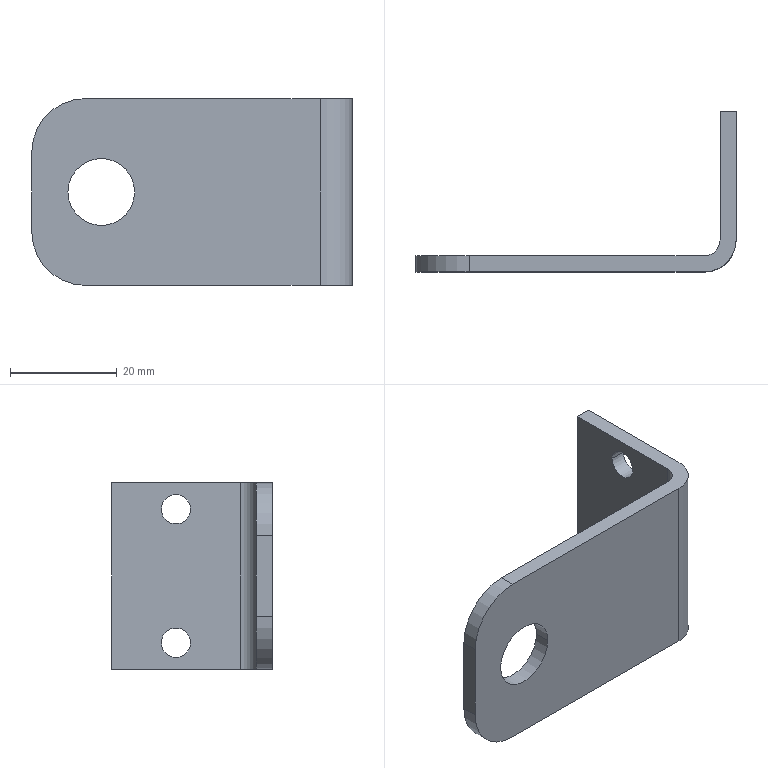Part | STEP file | X77-04022 | 1 solid | 18 faces | box 60 x 30 x 35 mm | volume 8293 mm3 | cylinder 10 | plane 8 | commonest cylinder face diameters 5.5 x4 12.5 x2 20 x2 6 x1 12 x1
STEP:
#1=CARTESIAN_POINT('',(-37.75,-30.,17.5));
#2=VERTEX_POINT('',#1);
#3=CARTESIAN_POINT('',(-50.25,-30.,17.5));
#4=VERTEX_POINT('',#3);
#5=CARTESIAN_POINT('',(-44.,-30.,17.5));
#6=DIRECTION('',(0.,1.,0.));
#7=DIRECTION('',(-1.,0.,0.));
#8=AXIS2_PLACEMENT_3D('',#5,#6,#7);
#9=CIRCLE('',#8,6.25);
#10=EDGE_CURVE('',#2,#4,#9,.T.);
#11=ORIENTED_EDGE('',*,*,#10,.F.);
#12=CARTESIAN_POINT('',(-37.75,-27.,17.5));
#13=VERTEX_POINT('',#12);
#14=CARTESIAN_POINT('',(-37.75,-30.,17.5));
#15=DIRECTION('',(0.,1.,0.));
#16=VECTOR('',#15,1000.);
#17=LINE('',#14,#16);
#18=EDGE_CURVE('',#2,#13,#17,.T.);
#19=ORIENTED_EDGE('',*,*,#18,.T.);
#20=CARTESIAN_POINT('',(-50.25,-27.,17.5));
#21=VERTEX_POINT('',#20);
#22=CARTESIAN_POINT('',(-44.,-27.,17.5));
#23=DIRECTION('',(0.,1.,0.));
#24=DIRECTION('',(-1.,0.,0.));
#25=AXIS2_PLACEMENT_3D('',#22,#23,#24);
#26=CIRCLE('',#25,6.25);
#27=EDGE_CURVE('',#13,#21,#26,.T.);
#28=ORIENTED_EDGE('',*,*,#27,.T.);
#29=CARTESIAN_POINT('',(-50.25,-30.,17.5));
#30=DIRECTION('',(0.,1.,0.));
#31=VECTOR('',#30,1000.);
#32=LINE('',#29,#31);
#33=EDGE_CURVE('',#4,#21,#32,.T.);
#34=ORIENTED_EDGE('',*,*,#33,.F.);
#35=EDGE_LOOP('',(#11,#19,#28,#34));
#36=FACE_OUTER_BOUND('',#35,.T.);
#37=CARTESIAN_POINT('',(-44.,-30.,17.5));
#38=DIRECTION('',(0.,1.,0.));
#39=DIRECTION('',(-1.,0.,0.));
#40=AXIS2_PLACEMENT_3D('',#37,#38,#39);
#41=CYLINDRICAL_SURFACE('',#40,6.25);
#42=ADVANCED_FACE('',(#36),#41,.F.);
#43=CARTESIAN_POINT('',(3.,-9.25,30.));
#44=VERTEX_POINT('',#43);
#45=CARTESIAN_POINT('',(3.,-14.75,30.));
#46=VERTEX_POINT('',#45);
#47=CARTESIAN_POINT('',(3.,-12.,30.));
#48=DIRECTION('',(-1.,0.,0.));
#49=DIRECTION('',(0.,-1.,0.));
#50=AXIS2_PLACEMENT_3D('',#47,#48,#49);
#51=CIRCLE('',#50,2.75);
#52=EDGE_CURVE('',#44,#46,#51,.T.);
#53=ORIENTED_EDGE('',*,*,#52,.F.);
#54=CARTESIAN_POINT('',(0.,-9.25,30.));
#55=VERTEX_POINT('',#54);
#56=CARTESIAN_POINT('',(3.,-9.25,30.));
#57=DIRECTION('',(-1.,0.,0.));
#58=VECTOR('',#57,1000.);
#59=LINE('',#56,#58);
#60=EDGE_CURVE('',#44,#55,#59,.T.);
#61=ORIENTED_EDGE('',*,*,#60,.T.);
#62=CARTESIAN_POINT('',(0.,-14.75,30.));
#63=VERTEX_POINT('',#62);
#64=CARTESIAN_POINT('',(0.,-12.,30.));
#65=DIRECTION('',(-1.,0.,0.));
#66=DIRECTION('',(0.,-1.,0.));
#67=AXIS2_PLACEMENT_3D('',#64,#65,#66);
#68=CIRCLE('',#67,2.75);
#69=EDGE_CURVE('',#55,#63,#68,.T.);
#70=ORIENTED_EDGE('',*,*,#69,.T.);
#71=CARTESIAN_POINT('',(3.,-14.75,30.));
#72=DIRECTION('',(-1.,0.,0.));
#73=VECTOR('',#72,1000.);
#74=LINE('',#71,#73);
#75=EDGE_CURVE('',#46,#63,#74,.T.);
#76=ORIENTED_EDGE('',*,*,#75,.F.);
#77=EDGE_LOOP('',(#53,#61,#70,#76));
#78=FACE_OUTER_BOUND('',#77,.T.);
#79=CARTESIAN_POINT('',(3.,-12.,30.));
#80=DIRECTION('',(-1.,0.,0.));
#81=DIRECTION('',(0.,-1.,0.));
#82=AXIS2_PLACEMENT_3D('',#79,#80,#81);
#83=CYLINDRICAL_SURFACE('',#82,2.75);
#84=ADVANCED_FACE('',(#78),#83,.F.);
#85=CARTESIAN_POINT('',(3.,-9.25,5.));
#86=VERTEX_POINT('',#85);
#87=CARTESIAN_POINT('',(3.,-14.75,5.));
#88=VERTEX_POINT('',#87);
#89=CARTESIAN_POINT('',(3.,-12.,5.));
#90=DIRECTION('',(-1.,0.,0.));
#91=DIRECTION('',(0.,-1.,0.));
#92=AXIS2_PLACEMENT_3D('',#89,#90,#91);
#93=CIRCLE('',#92,2.75);
#94=EDGE_CURVE('',#86,#88,#93,.T.);
#95=ORIENTED_EDGE('',*,*,#94,.F.);
#96=CARTESIAN_POINT('',(0.,-9.25,5.));
#97=VERTEX_POINT('',#96);
#98=CARTESIAN_POINT('',(3.,-9.25,5.));
#99=DIRECTION('',(-1.,0.,0.));
#100=VECTOR('',#99,1000.);
#101=LINE('',#98,#100);
#102=EDGE_CURVE('',#86,#97,#101,.T.);
#103=ORIENTED_EDGE('',*,*,#102,.T.);
#104=CARTESIAN_POINT('',(0.,-14.75,5.));
#105=VERTEX_POINT('',#104);
#106=CARTESIAN_POINT('',(0.,-12.,5.));
#107=DIRECTION('',(-1.,0.,0.));
#108=DIRECTION('',(0.,-1.,0.));
#109=AXIS2_PLACEMENT_3D('',#106,#107,#108);
#110=CIRCLE('',#109,2.75);
#111=EDGE_CURVE('',#97,#105,#110,.T.);
#112=ORIENTED_EDGE('',*,*,#111,.T.);
#113=CARTESIAN_POINT('',(3.,-14.75,5.));
#114=DIRECTION('',(-1.,0.,0.));
#115=VECTOR('',#114,1000.);
#116=LINE('',#113,#115);
#117=EDGE_CURVE('',#88,#105,#116,.T.);
#118=ORIENTED_EDGE('',*,*,#117,.F.);
#119=EDGE_LOOP('',(#95,#103,#112,#118));
#120=FACE_OUTER_BOUND('',#119,.T.);
#121=CARTESIAN_POINT('',(3.,-12.,5.));
#122=DIRECTION('',(-1.,0.,0.));
#123=DIRECTION('',(0.,-1.,0.));
#124=AXIS2_PLACEMENT_3D('',#121,#122,#123);
#125=CYLINDRICAL_SURFACE('',#124,2.75);
#126=ADVANCED_FACE('',(#120),#125,.F.);
#127=CARTESIAN_POINT('',(3.,0.,0.));
#128=VERTEX_POINT('',#127);
#129=CARTESIAN_POINT('',(0.,0.,0.));
#130=VERTEX_POINT('',#129);
#131=CARTESIAN_POINT('',(3.,0.,0.));
#132=DIRECTION('',(-1.,0.,0.));
#133=VECTOR('',#132,1000.);
#134=LINE('',#131,#133);
#135=EDGE_CURVE('',#128,#130,#134,.T.);
#136=ORIENTED_EDGE('',*,*,#135,.T.);
#137=CARTESIAN_POINT('',(0.,0.,35.));
#138=VERTEX_POINT('',#137);
#139=CARTESIAN_POINT('',(0.,0.,35.));
#140=DIRECTION('',(0.,0.,-1.));
#141=VECTOR('',#140,1000.);
#142=LINE('',#139,#141);
#143=EDGE_CURVE('',#138,#130,#142,.T.);
#144=ORIENTED_EDGE('',*,*,#143,.F.);
#145=CARTESIAN_POINT('',(3.,0.,35.));
#146=VERTEX_POINT('',#145);
#147=CARTESIAN_POINT('',(3.,0.,35.));
#148=DIRECTION('',(-1.,0.,0.));
#149=VECTOR('',#148,1000.);
#150=LINE('',#147,#149);
#151=EDGE_CURVE('',#146,#138,#150,.T.);
#152=ORIENTED_EDGE('',*,*,#151,.F.);
#153=CARTESIAN_POINT('',(3.,0.,35.));
#154=DIRECTION('',(0.,0.,-1.));
#155=VECTOR('',#154,1000.);
#156=LINE('',#153,#155);
#157=EDGE_CURVE('',#146,#128,#156,.T.);
#158=ORIENTED_EDGE('',*,*,#157,.T.);
#159=EDGE_LOOP('',(#136,#144,#152,#158));
#160=FACE_OUTER_BOUND('',#159,.T.);
#161=CARTESIAN_POINT('',(3.,0.,35.));
#162=DIRECTION('',(0.,-1.,0.));
#163=DIRECTION('',(1.,0.,0.));
#164=AXIS2_PLACEMENT_3D('',#161,#162,#163);
#165=PLANE('',#164);
#166=ADVANCED_FACE('',(#160),#165,.F.);
#167=CARTESIAN_POINT('',(0.,-12.,30.));
#168=DIRECTION('',(-1.,0.,0.));
#169=DIRECTION('',(0.,-1.,0.));
#170=AXIS2_PLACEMENT_3D('',#167,#168,#169);
#171=CIRCLE('',#170,2.75);
#172=EDGE_CURVE('',#63,#55,#171,.T.);
#173=ORIENTED_EDGE('',*,*,#172,.F.);
#174=ORIENTED_EDGE('',*,*,#69,.F.);
#175=EDGE_LOOP('',(#173,#174));
#176=FACE_BOUND('',#175,.T.);
#177=CARTESIAN_POINT('',(0.,-12.,5.));
#178=DIRECTION('',(-1.,0.,0.));
#179=DIRECTION('',(0.,-1.,0.));
#180=AXIS2_PLACEMENT_3D('',#177,#178,#179);
#181=CIRCLE('',#180,2.75);
#182=EDGE_CURVE('',#105,#97,#181,.T.);
#183=ORIENTED_EDGE('',*,*,#182,.F.);
#184=ORIENTED_EDGE('',*,*,#111,.F.);
#185=EDGE_LOOP('',(#183,#184));
#186=FACE_BOUND('',#185,.T.);
#187=CARTESIAN_POINT('',(0.,-24.,0.));
#188=VERTEX_POINT('',#187);
#189=CARTESIAN_POINT('',(0.,0.,0.));
#190=DIRECTION('',(0.,-1.,0.));
#191=VECTOR('',#190,1000.);
#192=LINE('',#189,#191);
#193=EDGE_CURVE('',#130,#188,#192,.T.);
#194=ORIENTED_EDGE('',*,*,#193,.T.);
#195=CARTESIAN_POINT('',(0.,-24.,35.));
#196=VERTEX_POINT('',#195);
#197=CARTESIAN_POINT('',(0.,-24.,35.));
#198=DIRECTION('',(0.,0.,-1.));
#199=VECTOR('',#198,1000.);
#200=LINE('',#197,#199);
#201=EDGE_CURVE('',#196,#188,#200,.T.);
#202=ORIENTED_EDGE('',*,*,#201,.F.);
#203=CARTESIAN_POINT('',(0.,0.,35.));
#204=DIRECTION('',(0.,-1.,0.));
#205=VECTOR('',#204,1000.);
#206=LINE('',#203,#205);
#207=EDGE_CURVE('',#138,#196,#206,.T.);
#208=ORIENTED_EDGE('',*,*,#207,.F.);
#209=ORIENTED_EDGE('',*,*,#143,.T.);
#210=EDGE_LOOP('',(#194,#202,#208,#209));
#211=FACE_OUTER_BOUND('',#210,.T.);
#212=CARTESIAN_POINT('',(0.,0.,35.));
#213=DIRECTION('',(1.,0.,0.));
#214=DIRECTION('',(0.,1.,0.));
#215=AXIS2_PLACEMENT_3D('',#212,#213,#214);
#216=PLANE('',#215);
#217=ADVANCED_FACE('',(#176,#186,#211),#216,.F.);
#218=CARTESIAN_POINT('',(-3.,-27.,0.));
#219=VERTEX_POINT('',#218);
#220=CARTESIAN_POINT('',(-3.,-24.,0.));
#221=DIRECTION('',(0.,0.,-1.));
#222=DIRECTION('',(1.,0.,0.));
#223=AXIS2_PLACEMENT_3D('',#220,#221,#222);
#224=CIRCLE('',#223,3.);
#225=EDGE_CURVE('',#188,#219,#224,.T.);
#226=ORIENTED_EDGE('',*,*,#225,.T.);
#227=CARTESIAN_POINT('',(-3.,-27.,35.));
#228=VERTEX_POINT('',#227);
#229=CARTESIAN_POINT('',(-3.,-27.,35.));
#230=DIRECTION('',(0.,0.,-1.));
#231=VECTOR('',#230,1000.);
#232=LINE('',#229,#231);
#233=EDGE_CURVE('',#228,#219,#232,.T.);
#234=ORIENTED_EDGE('',*,*,#233,.F.);
#235=CARTESIAN_POINT('',(-3.,-24.,35.));
#236=DIRECTION('',(0.,0.,-1.));
#237=DIRECTION('',(1.,0.,0.));
#238=AXIS2_PLACEMENT_3D('',#235,#236,#237);
#239=CIRCLE('',#238,3.);
#240=EDGE_CURVE('',#196,#228,#239,.T.);
#241=ORIENTED_EDGE('',*,*,#240,.F.);
#242=ORIENTED_EDGE('',*,*,#201,.T.);
#243=EDGE_LOOP('',(#226,#234,#241,#242));
#244=FACE_OUTER_BOUND('',#243,.T.);
#245=CARTESIAN_POINT('',(-3.,-24.,35.));
#246=DIRECTION('',(0.,0.,-1.));
#247=DIRECTION('',(-1.,0.,0.));
#248=AXIS2_PLACEMENT_3D('',#245,#246,#247);
#249=CYLINDRICAL_SURFACE('',#248,3.);
#250=ADVANCED_FACE('',(#244),#249,.F.);
#251=CARTESIAN_POINT('',(-44.,-27.,17.5));
#252=DIRECTION('',(0.,1.,0.));
#253=DIRECTION('',(-1.,0.,0.));
#254=AXIS2_PLACEMENT_3D('',#251,#252,#253);
#255=CIRCLE('',#254,6.25);
#256=EDGE_CURVE('',#21,#13,#255,.T.);
#257=ORIENTED_EDGE('',*,*,#256,.F.);
#258=ORIENTED_EDGE('',*,*,#27,.F.);
#259=EDGE_LOOP('',(#257,#258));
#260=FACE_BOUND('',#259,.T.);
#261=CARTESIAN_POINT('',(-57.,-27.,25.));
#262=VERTEX_POINT('',#261);
#263=CARTESIAN_POINT('',(-57.,-27.,10.));
#264=VERTEX_POINT('',#263);
#265=CARTESIAN_POINT('',(-57.,-27.,35.));
#266=DIRECTION('',(0.,0.,-1.));
#267=VECTOR('',#266,1000.);
#268=LINE('',#265,#267);
#269=EDGE_CURVE('',#262,#264,#268,.T.);
#270=ORIENTED_EDGE('',*,*,#269,.F.);
#271=CARTESIAN_POINT('',(-47.,-27.,35.));
#272=VERTEX_POINT('',#271);
#273=CARTESIAN_POINT('',(-47.,-27.,25.));
#274=DIRECTION('',(0.,1.,0.));
#275=DIRECTION('',(0.,0.,-1.));
#276=AXIS2_PLACEMENT_3D('',#273,#274,#275);
#277=CIRCLE('',#276,10.);
#278=EDGE_CURVE('',#262,#272,#277,.T.);
#279=ORIENTED_EDGE('',*,*,#278,.T.);
#280=CARTESIAN_POINT('',(-3.,-27.,35.));
#281=DIRECTION('',(-1.,0.,0.));
#282=VECTOR('',#281,1000.);
#283=LINE('',#280,#282);
#284=EDGE_CURVE('',#228,#272,#283,.T.);
#285=ORIENTED_EDGE('',*,*,#284,.F.);
#286=ORIENTED_EDGE('',*,*,#233,.T.);
#287=CARTESIAN_POINT('',(-47.,-27.,0.));
#288=VERTEX_POINT('',#287);
#289=CARTESIAN_POINT('',(-3.,-27.,0.));
#290=DIRECTION('',(-1.,0.,0.));
#291=VECTOR('',#290,1000.);
#292=LINE('',#289,#291);
#293=EDGE_CURVE('',#219,#288,#292,.T.);
#294=ORIENTED_EDGE('',*,*,#293,.T.);
#295=CARTESIAN_POINT('',(-47.,-27.,10.));
#296=DIRECTION('',(0.,1.,0.));
#297=DIRECTION('',(0.,0.,-1.));
#298=AXIS2_PLACEMENT_3D('',#295,#296,#297);
#299=CIRCLE('',#298,10.);
#300=EDGE_CURVE('',#288,#264,#299,.T.);
#301=ORIENTED_EDGE('',*,*,#300,.T.);
#302=EDGE_LOOP('',(#270,#279,#285,#286,#294,#301));
#303=FACE_OUTER_BOUND('',#302,.T.);
#304=CARTESIAN_POINT('',(-3.,-27.,35.));
#305=DIRECTION('',(0.,-1.,0.));
#306=DIRECTION('',(0.,0.,-1.));
#307=AXIS2_PLACEMENT_3D('',#304,#305,#306);
#308=PLANE('',#307);
#309=ADVANCED_FACE('',(#260,#303),#308,.F.);
#310=CARTESIAN_POINT('',(-57.,-30.,25.));
#311=VERTEX_POINT('',#310);
#312=CARTESIAN_POINT('',(-57.,-30.,10.));
#313=VERTEX_POINT('',#312);
#314=CARTESIAN_POINT('',(-57.,-30.,35.));
#315=DIRECTION('',(0.,0.,-1.));
#316=VECTOR('',#315,1000.);
#317=LINE('',#314,#316);
#318=EDGE_CURVE('',#311,#313,#317,.T.);
#319=ORIENTED_EDGE('',*,*,#318,.F.);
#320=CARTESIAN_POINT('',(-57.,-27.,25.));
#321=DIRECTION('',(0.,1.,0.));
#322=VECTOR('',#321,1000.);
#323=LINE('',#320,#322);
#324=EDGE_CURVE('',#311,#262,#323,.T.);
#325=ORIENTED_EDGE('',*,*,#324,.T.);
#326=ORIENTED_EDGE('',*,*,#269,.T.);
#327=CARTESIAN_POINT('',(-57.,-27.,10.));
#328=DIRECTION('',(0.,-1.,0.));
#329=VECTOR('',#328,1000.);
#330=LINE('',#327,#329);
#331=EDGE_CURVE('',#264,#313,#330,.T.);
#332=ORIENTED_EDGE('',*,*,#331,.T.);
#333=EDGE_LOOP('',(#319,#325,#326,#332));
#334=FACE_OUTER_BOUND('',#333,.T.);
#335=CARTESIAN_POINT('',(-57.,-27.,35.));
#336=DIRECTION('',(1.,0.,0.));
#337=DIRECTION('',(0.,0.,-1.));
#338=AXIS2_PLACEMENT_3D('',#335,#336,#337);
#339=PLANE('',#338);
#340=ADVANCED_FACE('',(#334),#339,.F.);
#341=CARTESIAN_POINT('',(-44.,-30.,17.5));
#342=DIRECTION('',(0.,1.,0.));
#343=DIRECTION('',(-1.,0.,0.));
#344=AXIS2_PLACEMENT_3D('',#341,#342,#343);
#345=CIRCLE('',#344,6.25);
#346=EDGE_CURVE('',#4,#2,#345,.T.);
#347=ORIENTED_EDGE('',*,*,#346,.T.);
#348=ORIENTED_EDGE('',*,*,#10,.T.);
#349=EDGE_LOOP('',(#347,#348));
#350=FACE_BOUND('',#349,.T.);
#351=CARTESIAN_POINT('',(-47.,-30.,35.));
#352=VERTEX_POINT('',#351);
#353=CARTESIAN_POINT('',(-3.,-30.,35.));
#354=VERTEX_POINT('',#353);
#355=CARTESIAN_POINT('',(-57.,-30.,35.));
#356=DIRECTION('',(1.,0.,0.));
#357=VECTOR('',#356,1000.);
#358=LINE('',#355,#357);
#359=EDGE_CURVE('',#352,#354,#358,.T.);
#360=ORIENTED_EDGE('',*,*,#359,.F.);
#361=CARTESIAN_POINT('',(-47.,-30.,25.));
#362=DIRECTION('',(0.,-1.,0.));
#363=DIRECTION('',(0.,0.,1.));
#364=AXIS2_PLACEMENT_3D('',#361,#362,#363);
#365=CIRCLE('',#364,10.);
#366=EDGE_CURVE('',#352,#311,#365,.T.);
#367=ORIENTED_EDGE('',*,*,#366,.T.);
#368=ORIENTED_EDGE('',*,*,#318,.T.);
#369=CARTESIAN_POINT('',(-47.,-30.,0.));
#370=VERTEX_POINT('',#369);
#371=CARTESIAN_POINT('',(-47.,-30.,10.));
#372=DIRECTION('',(0.,-1.,0.));
#373=DIRECTION('',(0.,0.,1.));
#374=AXIS2_PLACEMENT_3D('',#371,#372,#373);
#375=CIRCLE('',#374,10.);
#376=EDGE_CURVE('',#313,#370,#375,.T.);
#377=ORIENTED_EDGE('',*,*,#376,.T.);
#378=CARTESIAN_POINT('',(-3.,-30.,0.));
#379=VERTEX_POINT('',#378);
#380=CARTESIAN_POINT('',(-57.,-30.,0.));
#381=DIRECTION('',(1.,0.,0.));
#382=VECTOR('',#381,1000.);
#383=LINE('',#380,#382);
#384=EDGE_CURVE('',#370,#379,#383,.T.);
#385=ORIENTED_EDGE('',*,*,#384,.T.);
#386=CARTESIAN_POINT('',(-3.,-30.,35.));
#387=DIRECTION('',(0.,0.,-1.));
#388=VECTOR('',#387,1000.);
#389=LINE('',#386,#388);
#390=EDGE_CURVE('',#354,#379,#389,.T.);
#391=ORIENTED_EDGE('',*,*,#390,.F.);
#392=EDGE_LOOP('',(#360,#367,#368,#377,#385,#391));
#393=FACE_OUTER_BOUND('',#392,.T.);
#394=CARTESIAN_POINT('',(-57.,-30.,35.));
#395=DIRECTION('',(0.,1.,0.));
#396=DIRECTION('',(0.,0.,1.));
#397=AXIS2_PLACEMENT_3D('',#394,#395,#396);
#398=PLANE('',#397);
#399=ADVANCED_FACE('',(#350,#393),#398,.F.);
#400=CARTESIAN_POINT('',(3.,-24.,0.));
#401=VERTEX_POINT('',#400);
#402=CARTESIAN_POINT('',(-3.,-24.,0.));
#403=DIRECTION('',(0.,0.,1.));
#404=DIRECTION('',(1.,0.,0.));
#405=AXIS2_PLACEMENT_3D('',#402,#403,#404);
#406=CIRCLE('',#405,6.);
#407=EDGE_CURVE('',#379,#401,#406,.T.);
#408=ORIENTED_EDGE('',*,*,#407,.T.);
#409=CARTESIAN_POINT('',(3.,-24.,35.));
#410=VERTEX_POINT('',#409);
#411=CARTESIAN_POINT('',(3.,-24.,35.));
#412=DIRECTION('',(0.,0.,-1.));
#413=VECTOR('',#412,1000.);
#414=LINE('',#411,#413);
#415=EDGE_CURVE('',#410,#401,#414,.T.);
#416=ORIENTED_EDGE('',*,*,#415,.F.);
#417=CARTESIAN_POINT('',(-3.,-24.,35.));
#418=DIRECTION('',(0.,0.,1.));
#419=DIRECTION('',(1.,0.,0.));
#420=AXIS2_PLACEMENT_3D('',#417,#418,#419);
#421=CIRCLE('',#420,6.);
#422=EDGE_CURVE('',#354,#410,#421,.T.);
#423=ORIENTED_EDGE('',*,*,#422,.F.);
#424=ORIENTED_EDGE('',*,*,#390,.T.);
#425=EDGE_LOOP('',(#408,#416,#423,#424));
#426=FACE_OUTER_BOUND('',#425,.T.);
#427=CARTESIAN_POINT('',(-3.,-24.,35.));
#428=DIRECTION('',(0.,0.,-1.));
#429=DIRECTION('',(-1.,0.,0.));
#430=AXIS2_PLACEMENT_3D('',#427,#428,#429);
#431=CYLINDRICAL_SURFACE('',#430,6.);
#432=ADVANCED_FACE('',(#426),#431,.T.);
#433=CARTESIAN_POINT('',(3.,-12.,30.));
#434=DIRECTION('',(-1.,0.,0.));
#435=DIRECTION('',(0.,-1.,0.));
#436=AXIS2_PLACEMENT_3D('',#433,#434,#435);
#437=CIRCLE('',#436,2.75);
#438=EDGE_CURVE('',#46,#44,#437,.T.);
#439=ORIENTED_EDGE('',*,*,#438,.T.);
#440=ORIENTED_EDGE('',*,*,#52,.T.);
#441=EDGE_LOOP('',(#439,#440));
#442=FACE_BOUND('',#441,.T.);
#443=CARTESIAN_POINT('',(3.,-12.,5.));
#444=DIRECTION('',(-1.,0.,0.));
#445=DIRECTION('',(0.,-1.,0.));
#446=AXIS2_PLACEMENT_3D('',#443,#444,#445);
#447=CIRCLE('',#446,2.75);
#448=EDGE_CURVE('',#88,#86,#447,.T.);
#449=ORIENTED_EDGE('',*,*,#448,.T.);
#450=ORIENTED_EDGE('',*,*,#94,.T.);
#451=EDGE_LOOP('',(#449,#450));
#452=FACE_BOUND('',#451,.T.);
#453=CARTESIAN_POINT('',(3.,-24.,0.));
#454=DIRECTION('',(0.,1.,0.));
#455=VECTOR('',#454,1000.);
#456=LINE('',#453,#455);
#457=EDGE_CURVE('',#401,#128,#456,.T.);
#458=ORIENTED_EDGE('',*,*,#457,.T.);
#459=ORIENTED_EDGE('',*,*,#157,.F.);
#460=CARTESIAN_POINT('',(3.,-24.,35.));
#461=DIRECTION('',(0.,1.,0.));
#462=VECTOR('',#461,1000.);
#463=LINE('',#460,#462);
#464=EDGE_CURVE('',#410,#146,#463,.T.);
#465=ORIENTED_EDGE('',*,*,#464,.F.);
#466=ORIENTED_EDGE('',*,*,#415,.T.);
#467=EDGE_LOOP('',(#458,#459,#465,#466));
#468=FACE_OUTER_BOUND('',#467,.T.);
#469=CARTESIAN_POINT('',(3.,-24.,35.));
#470=DIRECTION('',(-1.,0.,0.));
#471=DIRECTION('',(0.,0.,1.));
#472=AXIS2_PLACEMENT_3D('',#469,#470,#471);
#473=PLANE('',#472);
#474=ADVANCED_FACE('',(#442,#452,#468),#473,.F.);
#475=ORIENTED_EDGE('',*,*,#284,.T.);
#476=CARTESIAN_POINT('',(-47.,-30.,35.));
#477=DIRECTION('',(0.,-1.,0.));
#478=VECTOR('',#477,1000.);
#479=LINE('',#476,#478);
#480=EDGE_CURVE('',#272,#352,#479,.T.);
#481=ORIENTED_EDGE('',*,*,#480,.T.);
#482=ORIENTED_EDGE('',*,*,#359,.T.);
#483=ORIENTED_EDGE('',*,*,#422,.T.);
#484=ORIENTED_EDGE('',*,*,#464,.T.);
#485=ORIENTED_EDGE('',*,*,#151,.T.);
#486=ORIENTED_EDGE('',*,*,#207,.T.);
#487=ORIENTED_EDGE('',*,*,#240,.T.);
#488=EDGE_LOOP('',(#475,#481,#482,#483,#484,#485,#486,#487));
#489=FACE_OUTER_BOUND('',#488,.T.);
#490=CARTESIAN_POINT('',(-3.,-24.,35.));
#491=DIRECTION('',(0.,0.,1.));
#492=DIRECTION('',(1.,0.,0.));
#493=AXIS2_PLACEMENT_3D('',#490,#491,#492);
#494=PLANE('',#493);
#495=ADVANCED_FACE('',(#489),#494,.T.);
#496=ORIENTED_EDGE('',*,*,#384,.F.);
#497=CARTESIAN_POINT('',(-47.,-24.,0.));
#498=DIRECTION('',(0.,1.,0.));
#499=VECTOR('',#498,1000.);
#500=LINE('',#497,#499);
#501=EDGE_CURVE('',#370,#288,#500,.T.);
#502=ORIENTED_EDGE('',*,*,#501,.T.);
#503=ORIENTED_EDGE('',*,*,#293,.F.);
#504=ORIENTED_EDGE('',*,*,#225,.F.);
#505=ORIENTED_EDGE('',*,*,#193,.F.);
#506=ORIENTED_EDGE('',*,*,#135,.F.);
#507=ORIENTED_EDGE('',*,*,#457,.F.);
#508=ORIENTED_EDGE('',*,*,#407,.F.);
#509=EDGE_LOOP('',(#496,#502,#503,#504,#505,#506,#507,#508));
#510=FACE_OUTER_BOUND('',#509,.T.);
#511=CARTESIAN_POINT('',(-3.,-24.,0.));
#512=DIRECTION('',(0.,0.,1.));
#513=DIRECTION('',(1.,0.,0.));
#514=AXIS2_PLACEMENT_3D('',#511,#512,#513);
#515=PLANE('',#514);
#516=ADVANCED_FACE('',(#510),#515,.F.);
#517=ORIENTED_EDGE('',*,*,#102,.F.);
#518=ORIENTED_EDGE('',*,*,#448,.F.);
#519=ORIENTED_EDGE('',*,*,#117,.T.);
#520=ORIENTED_EDGE('',*,*,#182,.T.);
#521=EDGE_LOOP('',(#517,#518,#519,#520));
#522=FACE_OUTER_BOUND('',#521,.T.);
#523=CARTESIAN_POINT('',(3.,-12.,5.));
#524=DIRECTION('',(-1.,0.,0.));
#525=DIRECTION('',(0.,-1.,0.));
#526=AXIS2_PLACEMENT_3D('',#523,#524,#525);
#527=CYLINDRICAL_SURFACE('',#526,2.75);
#528=ADVANCED_FACE('',(#522),#527,.F.);
#529=ORIENTED_EDGE('',*,*,#60,.F.);
#530=ORIENTED_EDGE('',*,*,#438,.F.);
#531=ORIENTED_EDGE('',*,*,#75,.T.);
#532=ORIENTED_EDGE('',*,*,#172,.T.);
#533=EDGE_LOOP('',(#529,#530,#531,#532));
#534=FACE_OUTER_BOUND('',#533,.T.);
#535=CARTESIAN_POINT('',(3.,-12.,30.));
#536=DIRECTION('',(-1.,0.,0.));
#537=DIRECTION('',(0.,-1.,0.));
#538=AXIS2_PLACEMENT_3D('',#535,#536,#537);
#539=CYLINDRICAL_SURFACE('',#538,2.75);
#540=ADVANCED_FACE('',(#534),#539,.F.);
#541=ORIENTED_EDGE('',*,*,#18,.F.);
#542=ORIENTED_EDGE('',*,*,#346,.F.);
#543=ORIENTED_EDGE('',*,*,#33,.T.);
#544=ORIENTED_EDGE('',*,*,#256,.T.);
#545=EDGE_LOOP('',(#541,#542,#543,#544));
#546=FACE_OUTER_BOUND('',#545,.T.);
#547=CARTESIAN_POINT('',(-44.,-30.,17.5));
#548=DIRECTION('',(0.,1.,0.));
#549=DIRECTION('',(-1.,0.,0.));
#550=AXIS2_PLACEMENT_3D('',#547,#548,#549);
#551=CYLINDRICAL_SURFACE('',#550,6.25);
#552=ADVANCED_FACE('',(#546),#551,.F.);
#553=ORIENTED_EDGE('',*,*,#278,.F.);
#554=ORIENTED_EDGE('',*,*,#324,.F.);
#555=ORIENTED_EDGE('',*,*,#366,.F.);
#556=ORIENTED_EDGE('',*,*,#480,.F.);
#557=EDGE_LOOP('',(#553,#554,#555,#556));
#558=FACE_OUTER_BOUND('',#557,.T.);
#559=CARTESIAN_POINT('',(-47.,-24.,25.));
#560=DIRECTION('',(0.,1.,0.));
#561=DIRECTION('',(0.,0.,1.));
#562=AXIS2_PLACEMENT_3D('',#559,#560,#561);
#563=CYLINDRICAL_SURFACE('',#562,10.);
#564=ADVANCED_FACE('',(#558),#563,.T.);
#565=ORIENTED_EDGE('',*,*,#300,.F.);
#566=ORIENTED_EDGE('',*,*,#501,.F.);
#567=ORIENTED_EDGE('',*,*,#376,.F.);
#568=ORIENTED_EDGE('',*,*,#331,.F.);
#569=EDGE_LOOP('',(#565,#566,#567,#568));
#570=FACE_OUTER_BOUND('',#569,.T.);
#571=CARTESIAN_POINT('',(-47.,-27.,10.));
#572=DIRECTION('',(0.,-1.,0.));
#573=DIRECTION('',(0.,0.,-1.));
#574=AXIS2_PLACEMENT_3D('',#571,#572,#573);
#575=CYLINDRICAL_SURFACE('',#574,10.);
#576=ADVANCED_FACE('',(#570),#575,.T.);
#577=CLOSED_SHELL('',(#42,#84,#126,#166,#217,#250,#309,#340,#399,#432,#474,#495,#516,#528,#540,#552,#564,#576));
#578=MANIFOLD_SOLID_BREP('',#577);
#579=CARTESIAN_POINT('',(0.,0.,0.));
#580=DIRECTION('',(0.,0.,1.));
#581=DIRECTION('',(1.,0.,0.));
#582=AXIS2_PLACEMENT_3D('',#579,#580,#581);
#583=(LENGTH_UNIT()NAMED_UNIT(*)SI_UNIT(.MILLI.,.METRE.));
#584=UNCERTAINTY_MEASURE_WITH_UNIT(LENGTH_MEASURE(0.00001),#583,'','');
#585=(NAMED_UNIT(*)PLANE_ANGLE_UNIT()SI_UNIT($,.RADIAN.));
#586=(NAMED_UNIT(*)SI_UNIT($,.STERADIAN.)SOLID_ANGLE_UNIT());
#587=(GEOMETRIC_REPRESENTATION_CONTEXT(3)GLOBAL_UNCERTAINTY_ASSIGNED_CONTEXT((#584))GLOBAL_UNIT_ASSIGNED_CONTEXT((#583,#585,#586))REPRESENTATION_CONTEXT('',''));
#588=ADVANCED_BREP_SHAPE_REPRESENTATION('',(#578,#582),#587);